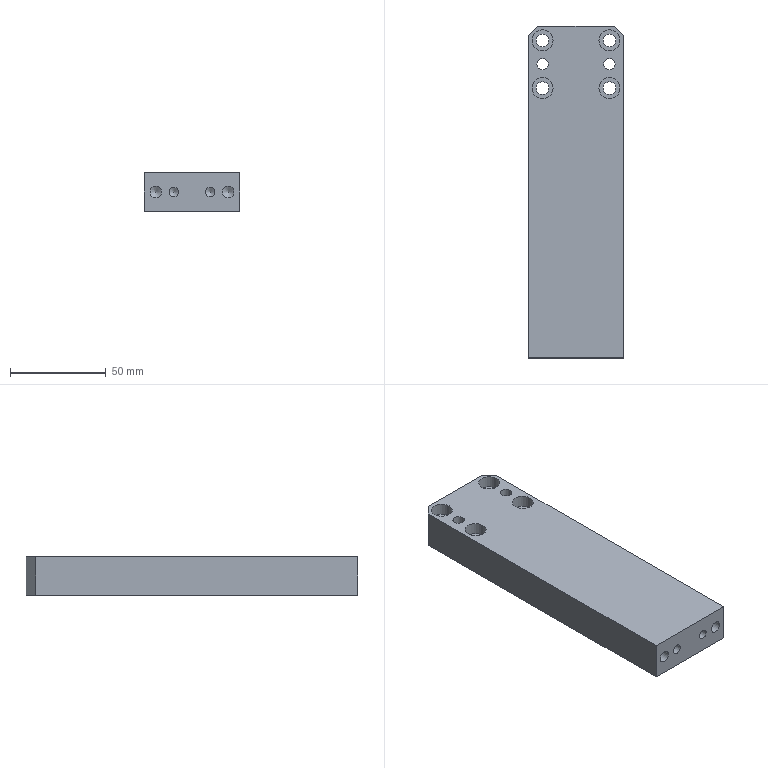Part | NX | features BREP 1 | 1 solid | 30 faces | box 50 x 173.75 x 20 mm | volume 166504 mm3 | cylinder 14 | plane 12 | cone 4 | commonest cylinder face diameters 6 x4 6.6 x4 11 x4 5 x2
STEP:
#1=CARTESIAN_POINT('',(25.,81.875,0.));
#2=VERTEX_POINT('',#1);
#3=CARTESIAN_POINT('',(20.,86.875,0.));
#4=VERTEX_POINT('',#3);
#5=CARTESIAN_POINT('',(25.,81.875,0.));
#6=DIRECTION('',(-0.7071,0.7071,0.));
#7=VECTOR('',#6,1000.);
#8=LINE('',#5,#7);
#9=EDGE_CURVE('',#2,#4,#8,.T.);
#10=ORIENTED_EDGE('',*,*,#9,.F.);
#11=CARTESIAN_POINT('',(25.,-86.875,0.));
#12=VERTEX_POINT('',#11);
#13=CARTESIAN_POINT('',(25.,0.,0.));
#14=DIRECTION('',(0.,1.,0.));
#15=VECTOR('',#14,1000.);
#16=LINE('',#13,#15);
#17=EDGE_CURVE('',#12,#2,#16,.T.);
#18=ORIENTED_EDGE('',*,*,#17,.F.);
#19=CARTESIAN_POINT('',(-25.,-86.875,0.));
#20=VERTEX_POINT('',#19);
#21=CARTESIAN_POINT('',(0.,-86.875,0.));
#22=DIRECTION('',(1.,0.,0.));
#23=VECTOR('',#22,1000.);
#24=LINE('',#21,#23);
#25=EDGE_CURVE('',#20,#12,#24,.T.);
#26=ORIENTED_EDGE('',*,*,#25,.F.);
#27=CARTESIAN_POINT('',(-25.,81.875,0.));
#28=VERTEX_POINT('',#27);
#29=CARTESIAN_POINT('',(-25.,0.,0.));
#30=DIRECTION('',(0.,-1.,0.));
#31=VECTOR('',#30,1000.);
#32=LINE('',#29,#31);
#33=EDGE_CURVE('',#28,#20,#32,.T.);
#34=ORIENTED_EDGE('',*,*,#33,.F.);
#35=CARTESIAN_POINT('',(-20.,86.875,0.));
#36=VERTEX_POINT('',#35);
#37=CARTESIAN_POINT('',(-20.,86.875,0.));
#38=DIRECTION('',(-0.7071,-0.7071,0.));
#39=VECTOR('',#38,1000.);
#40=LINE('',#37,#39);
#41=EDGE_CURVE('',#36,#28,#40,.T.);
#42=ORIENTED_EDGE('',*,*,#41,.F.);
#43=CARTESIAN_POINT('',(0.,86.875,0.));
#44=DIRECTION('',(-1.,0.,0.));
#45=VECTOR('',#44,1000.);
#46=LINE('',#43,#45);
#47=EDGE_CURVE('',#4,#36,#46,.T.);
#48=ORIENTED_EDGE('',*,*,#47,.F.);
#49=EDGE_LOOP('',(#10,#18,#26,#34,#42,#48));
#50=FACE_BOUND('',#49,.T.);
#51=CARTESIAN_POINT('',(14.5,66.875,0.));
#52=VERTEX_POINT('',#51);
#53=CARTESIAN_POINT('',(17.5,66.875,0.));
#54=DIRECTION('',(0.,0.,-1.));
#55=DIRECTION('',(-1.,0.,0.));
#56=AXIS2_PLACEMENT_3D('',#53,#54,#55);
#57=CIRCLE('',#56,3.);
#58=EDGE_CURVE('',#52,#52,#57,.T.);
#59=ORIENTED_EDGE('',*,*,#58,.F.);
#60=EDGE_LOOP('',(#59));
#61=FACE_BOUND('',#60,.T.);
#62=CARTESIAN_POINT('',(-20.5,66.875,0.));
#63=VERTEX_POINT('',#62);
#64=CARTESIAN_POINT('',(-17.5,66.875,0.));
#65=DIRECTION('',(0.,0.,-1.));
#66=DIRECTION('',(-1.,0.,0.));
#67=AXIS2_PLACEMENT_3D('',#64,#65,#66);
#68=CIRCLE('',#67,3.);
#69=EDGE_CURVE('',#63,#63,#68,.T.);
#70=ORIENTED_EDGE('',*,*,#69,.F.);
#71=EDGE_LOOP('',(#70));
#72=FACE_BOUND('',#71,.T.);
#73=CARTESIAN_POINT('',(20.8,54.375,0.));
#74=VERTEX_POINT('',#73);
#75=CARTESIAN_POINT('',(17.5,54.375,0.));
#76=DIRECTION('',(0.,0.,-1.));
#77=DIRECTION('',(1.,0.,0.));
#78=AXIS2_PLACEMENT_3D('',#75,#76,#77);
#79=CIRCLE('',#78,3.3);
#80=EDGE_CURVE('',#74,#74,#79,.T.);
#81=ORIENTED_EDGE('',*,*,#80,.F.);
#82=EDGE_LOOP('',(#81));
#83=FACE_BOUND('',#82,.T.);
#84=CARTESIAN_POINT('',(20.8,79.375,0.));
#85=VERTEX_POINT('',#84);
#86=CARTESIAN_POINT('',(17.5,79.375,0.));
#87=DIRECTION('',(0.,0.,-1.));
#88=DIRECTION('',(1.,0.,0.));
#89=AXIS2_PLACEMENT_3D('',#86,#87,#88);
#90=CIRCLE('',#89,3.3);
#91=EDGE_CURVE('',#85,#85,#90,.T.);
#92=ORIENTED_EDGE('',*,*,#91,.F.);
#93=EDGE_LOOP('',(#92));
#94=FACE_BOUND('',#93,.T.);
#95=CARTESIAN_POINT('',(-14.2,54.375,0.));
#96=VERTEX_POINT('',#95);
#97=CARTESIAN_POINT('',(-17.5,54.375,0.));
#98=DIRECTION('',(0.,0.,-1.));
#99=DIRECTION('',(1.,0.,0.));
#100=AXIS2_PLACEMENT_3D('',#97,#98,#99);
#101=CIRCLE('',#100,3.3);
#102=EDGE_CURVE('',#96,#96,#101,.T.);
#103=ORIENTED_EDGE('',*,*,#102,.F.);
#104=EDGE_LOOP('',(#103));
#105=FACE_BOUND('',#104,.T.);
#106=CARTESIAN_POINT('',(-14.2,79.375,0.));
#107=VERTEX_POINT('',#106);
#108=CARTESIAN_POINT('',(-17.5,79.375,0.));
#109=DIRECTION('',(0.,0.,-1.));
#110=DIRECTION('',(1.,0.,0.));
#111=AXIS2_PLACEMENT_3D('',#108,#109,#110);
#112=CIRCLE('',#111,3.3);
#113=EDGE_CURVE('',#107,#107,#112,.T.);
#114=ORIENTED_EDGE('',*,*,#113,.F.);
#115=EDGE_LOOP('',(#114));
#116=FACE_BOUND('',#115,.T.);
#117=CARTESIAN_POINT('',(0.,0.,0.));
#118=DIRECTION('',(0.,0.,1.));
#119=DIRECTION('',(-1.,0.,0.));
#120=AXIS2_PLACEMENT_3D('',#117,#118,#119);
#121=PLANE('',#120);
#122=ADVANCED_FACE('',(#50,#61,#72,#83,#94,#105,#116),#121,.F.);
#123=CARTESIAN_POINT('',(20.,86.875,20.));
#124=VERTEX_POINT('',#123);
#125=CARTESIAN_POINT('',(20.,86.875,20.));
#126=DIRECTION('',(0.,0.,1.));
#127=VECTOR('',#126,1000.);
#128=LINE('',#125,#127);
#129=EDGE_CURVE('',#4,#124,#128,.T.);
#130=ORIENTED_EDGE('',*,*,#129,.F.);
#131=ORIENTED_EDGE('',*,*,#47,.T.);
#132=CARTESIAN_POINT('',(-20.,86.875,20.));
#133=VERTEX_POINT('',#132);
#134=CARTESIAN_POINT('',(-20.,86.875,20.));
#135=DIRECTION('',(0.,0.,-1.));
#136=VECTOR('',#135,1000.);
#137=LINE('',#134,#136);
#138=EDGE_CURVE('',#133,#36,#137,.T.);
#139=ORIENTED_EDGE('',*,*,#138,.F.);
#140=CARTESIAN_POINT('',(-25.,86.875,20.));
#141=DIRECTION('',(-1.,0.,0.));
#142=VECTOR('',#141,1000.);
#143=LINE('',#140,#142);
#144=EDGE_CURVE('',#124,#133,#143,.T.);
#145=ORIENTED_EDGE('',*,*,#144,.F.);
#146=EDGE_LOOP('',(#130,#131,#139,#145));
#147=FACE_BOUND('',#146,.T.);
#148=CARTESIAN_POINT('',(-25.,86.875,20.));
#149=DIRECTION('',(0.,-1.,0.));
#150=DIRECTION('',(0.,0.,1.));
#151=AXIS2_PLACEMENT_3D('',#148,#149,#150);
#152=PLANE('',#151);
#153=ADVANCED_FACE('',(#147),#152,.F.);
#154=CARTESIAN_POINT('',(25.,81.875,20.));
#155=VERTEX_POINT('',#154);
#156=CARTESIAN_POINT('',(25.,81.875,20.));
#157=DIRECTION('',(0.,0.,1.));
#158=VECTOR('',#157,1000.);
#159=LINE('',#156,#158);
#160=EDGE_CURVE('',#2,#155,#159,.T.);
#161=ORIENTED_EDGE('',*,*,#160,.F.);
#162=ORIENTED_EDGE('',*,*,#9,.T.);
#163=ORIENTED_EDGE('',*,*,#129,.T.);
#164=CARTESIAN_POINT('',(20.,86.875,20.));
#165=DIRECTION('',(-0.7071,0.7071,0.));
#166=VECTOR('',#165,1000.);
#167=LINE('',#164,#166);
#168=EDGE_CURVE('',#155,#124,#167,.T.);
#169=ORIENTED_EDGE('',*,*,#168,.F.);
#170=EDGE_LOOP('',(#161,#162,#163,#169));
#171=FACE_BOUND('',#170,.T.);
#172=CARTESIAN_POINT('',(20.,86.875,20.));
#173=DIRECTION('',(-0.7071,-0.7071,0.));
#174=DIRECTION('',(-0.7071,0.7071,0.));
#175=AXIS2_PLACEMENT_3D('',#172,#173,#174);
#176=PLANE('',#175);
#177=ADVANCED_FACE('',(#171),#176,.F.);
#178=ORIENTED_EDGE('',*,*,#160,.T.);
#179=CARTESIAN_POINT('',(25.,-86.875,20.));
#180=VERTEX_POINT('',#179);
#181=CARTESIAN_POINT('',(25.,86.875,20.));
#182=DIRECTION('',(0.,1.,0.));
#183=VECTOR('',#182,1000.);
#184=LINE('',#181,#183);
#185=EDGE_CURVE('',#180,#155,#184,.T.);
#186=ORIENTED_EDGE('',*,*,#185,.F.);
#187=CARTESIAN_POINT('',(25.,-86.875,20.));
#188=DIRECTION('',(0.,0.,1.));
#189=VECTOR('',#188,1000.);
#190=LINE('',#187,#189);
#191=EDGE_CURVE('',#12,#180,#190,.T.);
#192=ORIENTED_EDGE('',*,*,#191,.F.);
#193=ORIENTED_EDGE('',*,*,#17,.T.);
#194=EDGE_LOOP('',(#178,#186,#192,#193));
#195=FACE_BOUND('',#194,.T.);
#196=CARTESIAN_POINT('',(25.,86.875,20.));
#197=DIRECTION('',(-1.,0.,0.));
#198=DIRECTION('',(0.,1.,0.));
#199=AXIS2_PLACEMENT_3D('',#196,#197,#198);
#200=PLANE('',#199);
#201=ADVANCED_FACE('',(#195),#200,.F.);
#202=ORIENTED_EDGE('',*,*,#191,.T.);
#203=CARTESIAN_POINT('',(-25.,-86.875,20.));
#204=VERTEX_POINT('',#203);
#205=CARTESIAN_POINT('',(-25.,-86.875,20.));
#206=DIRECTION('',(1.,0.,0.));
#207=VECTOR('',#206,1000.);
#208=LINE('',#205,#207);
#209=EDGE_CURVE('',#204,#180,#208,.T.);
#210=ORIENTED_EDGE('',*,*,#209,.F.);
#211=CARTESIAN_POINT('',(-25.,-86.875,20.));
#212=DIRECTION('',(0.,0.,1.));
#213=VECTOR('',#212,1000.);
#214=LINE('',#211,#213);
#215=EDGE_CURVE('',#20,#204,#214,.T.);
#216=ORIENTED_EDGE('',*,*,#215,.F.);
#217=ORIENTED_EDGE('',*,*,#25,.T.);
#218=EDGE_LOOP('',(#202,#210,#216,#217));
#219=FACE_BOUND('',#218,.T.);
#220=CARTESIAN_POINT('',(19.,-86.875,7.));
#221=VERTEX_POINT('',#220);
#222=CARTESIAN_POINT('',(19.,-86.875,10.));
#223=DIRECTION('',(0.,-1.,0.));
#224=DIRECTION('',(0.,0.,-1.));
#225=AXIS2_PLACEMENT_3D('',#222,#223,#224);
#226=CIRCLE('',#225,3.);
#227=EDGE_CURVE('',#221,#221,#226,.T.);
#228=ORIENTED_EDGE('',*,*,#227,.F.);
#229=EDGE_LOOP('',(#228));
#230=FACE_BOUND('',#229,.T.);
#231=CARTESIAN_POINT('',(-19.,-86.875,7.));
#232=VERTEX_POINT('',#231);
#233=CARTESIAN_POINT('',(-19.,-86.875,10.));
#234=DIRECTION('',(0.,-1.,0.));
#235=DIRECTION('',(0.,0.,-1.));
#236=AXIS2_PLACEMENT_3D('',#233,#234,#235);
#237=CIRCLE('',#236,3.);
#238=EDGE_CURVE('',#232,#232,#237,.T.);
#239=ORIENTED_EDGE('',*,*,#238,.F.);
#240=EDGE_LOOP('',(#239));
#241=FACE_BOUND('',#240,.T.);
#242=CARTESIAN_POINT('',(9.5,-86.875,7.5));
#243=VERTEX_POINT('',#242);
#244=CARTESIAN_POINT('',(9.5,-86.875,10.));
#245=DIRECTION('',(0.,-1.,0.));
#246=DIRECTION('',(0.,0.,-1.));
#247=AXIS2_PLACEMENT_3D('',#244,#245,#246);
#248=CIRCLE('',#247,2.5);
#249=EDGE_CURVE('',#243,#243,#248,.T.);
#250=ORIENTED_EDGE('',*,*,#249,.F.);
#251=EDGE_LOOP('',(#250));
#252=FACE_BOUND('',#251,.T.);
#253=CARTESIAN_POINT('',(-9.5,-86.875,7.5));
#254=VERTEX_POINT('',#253);
#255=CARTESIAN_POINT('',(-9.5,-86.875,10.));
#256=DIRECTION('',(0.,-1.,0.));
#257=DIRECTION('',(0.,0.,-1.));
#258=AXIS2_PLACEMENT_3D('',#255,#256,#257);
#259=CIRCLE('',#258,2.5);
#260=EDGE_CURVE('',#254,#254,#259,.T.);
#261=ORIENTED_EDGE('',*,*,#260,.F.);
#262=EDGE_LOOP('',(#261));
#263=FACE_BOUND('',#262,.T.);
#264=CARTESIAN_POINT('',(-25.,-86.875,20.));
#265=DIRECTION('',(0.,1.,0.));
#266=DIRECTION('',(0.,0.,-1.));
#267=AXIS2_PLACEMENT_3D('',#264,#265,#266);
#268=PLANE('',#267);
#269=ADVANCED_FACE('',(#219,#230,#241,#252,#263),#268,.F.);
#270=CARTESIAN_POINT('',(-25.,81.875,20.));
#271=VERTEX_POINT('',#270);
#272=CARTESIAN_POINT('',(-25.,81.875,20.));
#273=DIRECTION('',(0.,0.,1.));
#274=VECTOR('',#273,1000.);
#275=LINE('',#272,#274);
#276=EDGE_CURVE('',#28,#271,#275,.T.);
#277=ORIENTED_EDGE('',*,*,#276,.F.);
#278=ORIENTED_EDGE('',*,*,#33,.T.);
#279=ORIENTED_EDGE('',*,*,#215,.T.);
#280=CARTESIAN_POINT('',(-25.,86.875,20.));
#281=DIRECTION('',(0.,-1.,0.));
#282=VECTOR('',#281,1000.);
#283=LINE('',#280,#282);
#284=EDGE_CURVE('',#271,#204,#283,.T.);
#285=ORIENTED_EDGE('',*,*,#284,.F.);
#286=EDGE_LOOP('',(#277,#278,#279,#285));
#287=FACE_BOUND('',#286,.T.);
#288=CARTESIAN_POINT('',(-25.,86.875,20.));
#289=DIRECTION('',(1.,0.,0.));
#290=DIRECTION('',(0.,-1.,0.));
#291=AXIS2_PLACEMENT_3D('',#288,#289,#290);
#292=PLANE('',#291);
#293=ADVANCED_FACE('',(#287),#292,.F.);
#294=ORIENTED_EDGE('',*,*,#138,.T.);
#295=ORIENTED_EDGE('',*,*,#41,.T.);
#296=ORIENTED_EDGE('',*,*,#276,.T.);
#297=CARTESIAN_POINT('',(-25.,81.875,20.));
#298=DIRECTION('',(-0.7071,-0.7071,0.));
#299=VECTOR('',#298,1000.);
#300=LINE('',#297,#299);
#301=EDGE_CURVE('',#133,#271,#300,.T.);
#302=ORIENTED_EDGE('',*,*,#301,.F.);
#303=EDGE_LOOP('',(#294,#295,#296,#302));
#304=FACE_BOUND('',#303,.T.);
#305=CARTESIAN_POINT('',(-25.,81.875,20.));
#306=DIRECTION('',(0.7071,-0.7071,0.));
#307=DIRECTION('',(-0.7071,-0.7071,0.));
#308=AXIS2_PLACEMENT_3D('',#305,#306,#307);
#309=PLANE('',#308);
#310=ADVANCED_FACE('',(#304),#309,.F.);
#311=CARTESIAN_POINT('',(14.5,66.875,20.));
#312=VERTEX_POINT('',#311);
#313=CARTESIAN_POINT('',(17.5,66.875,20.));
#314=DIRECTION('',(0.,0.,-1.));
#315=DIRECTION('',(-1.,0.,0.));
#316=AXIS2_PLACEMENT_3D('',#313,#314,#315);
#317=CIRCLE('',#316,3.);
#318=EDGE_CURVE('',#312,#312,#317,.T.);
#319=ORIENTED_EDGE('',*,*,#318,.F.);
#320=EDGE_LOOP('',(#319));
#321=FACE_BOUND('',#320,.T.);
#322=ORIENTED_EDGE('',*,*,#58,.T.);
#323=EDGE_LOOP('',(#322));
#324=FACE_BOUND('',#323,.T.);
#325=CARTESIAN_POINT('',(17.5,66.875,0.));
#326=DIRECTION('',(0.,0.,-1.));
#327=DIRECTION('',(1.,0.,0.));
#328=AXIS2_PLACEMENT_3D('',#325,#326,#327);
#329=CYLINDRICAL_SURFACE('',#328,3.);
#330=ADVANCED_FACE('',(#321,#324),#329,.F.);
#331=CARTESIAN_POINT('',(-20.5,66.875,20.));
#332=VERTEX_POINT('',#331);
#333=CARTESIAN_POINT('',(-17.5,66.875,20.));
#334=DIRECTION('',(0.,0.,-1.));
#335=DIRECTION('',(-1.,0.,0.));
#336=AXIS2_PLACEMENT_3D('',#333,#334,#335);
#337=CIRCLE('',#336,3.);
#338=EDGE_CURVE('',#332,#332,#337,.T.);
#339=ORIENTED_EDGE('',*,*,#338,.F.);
#340=EDGE_LOOP('',(#339));
#341=FACE_BOUND('',#340,.T.);
#342=ORIENTED_EDGE('',*,*,#69,.T.);
#343=EDGE_LOOP('',(#342));
#344=FACE_BOUND('',#343,.T.);
#345=CARTESIAN_POINT('',(-17.5,66.875,0.));
#346=DIRECTION('',(0.,0.,-1.));
#347=DIRECTION('',(1.,0.,0.));
#348=AXIS2_PLACEMENT_3D('',#345,#346,#347);
#349=CYLINDRICAL_SURFACE('',#348,3.);
#350=ADVANCED_FACE('',(#341,#344),#349,.F.);
#351=ORIENTED_EDGE('',*,*,#80,.T.);
#352=EDGE_LOOP('',(#351));
#353=FACE_BOUND('',#352,.T.);
#354=CARTESIAN_POINT('',(20.8,54.375,13.6));
#355=VERTEX_POINT('',#354);
#356=CARTESIAN_POINT('',(17.5,54.375,13.6));
#357=DIRECTION('',(0.,0.,-1.));
#358=DIRECTION('',(1.,0.,0.));
#359=AXIS2_PLACEMENT_3D('',#356,#357,#358);
#360=CIRCLE('',#359,3.3);
#361=EDGE_CURVE('',#355,#355,#360,.T.);
#362=ORIENTED_EDGE('',*,*,#361,.F.);
#363=EDGE_LOOP('',(#362));
#364=FACE_BOUND('',#363,.T.);
#365=CARTESIAN_POINT('',(17.5,54.375,20.));
#366=DIRECTION('',(0.,0.,1.));
#367=DIRECTION('',(-1.,0.,0.));
#368=AXIS2_PLACEMENT_3D('',#365,#366,#367);
#369=CYLINDRICAL_SURFACE('',#368,3.3);
#370=ADVANCED_FACE('',(#353,#364),#369,.F.);
#371=ORIENTED_EDGE('',*,*,#91,.T.);
#372=EDGE_LOOP('',(#371));
#373=FACE_BOUND('',#372,.T.);
#374=CARTESIAN_POINT('',(20.8,79.375,13.6));
#375=VERTEX_POINT('',#374);
#376=CARTESIAN_POINT('',(17.5,79.375,13.6));
#377=DIRECTION('',(0.,0.,-1.));
#378=DIRECTION('',(1.,0.,0.));
#379=AXIS2_PLACEMENT_3D('',#376,#377,#378);
#380=CIRCLE('',#379,3.3);
#381=EDGE_CURVE('',#375,#375,#380,.T.);
#382=ORIENTED_EDGE('',*,*,#381,.F.);
#383=EDGE_LOOP('',(#382));
#384=FACE_BOUND('',#383,.T.);
#385=CARTESIAN_POINT('',(17.5,79.375,20.));
#386=DIRECTION('',(0.,0.,1.));
#387=DIRECTION('',(-1.,0.,0.));
#388=AXIS2_PLACEMENT_3D('',#385,#386,#387);
#389=CYLINDRICAL_SURFACE('',#388,3.3);
#390=ADVANCED_FACE('',(#373,#384),#389,.F.);
#391=ORIENTED_EDGE('',*,*,#102,.T.);
#392=EDGE_LOOP('',(#391));
#393=FACE_BOUND('',#392,.T.);
#394=CARTESIAN_POINT('',(-14.2,54.375,13.6));
#395=VERTEX_POINT('',#394);
#396=CARTESIAN_POINT('',(-17.5,54.375,13.6));
#397=DIRECTION('',(0.,0.,-1.));
#398=DIRECTION('',(1.,0.,0.));
#399=AXIS2_PLACEMENT_3D('',#396,#397,#398);
#400=CIRCLE('',#399,3.3);
#401=EDGE_CURVE('',#395,#395,#400,.T.);
#402=ORIENTED_EDGE('',*,*,#401,.F.);
#403=EDGE_LOOP('',(#402));
#404=FACE_BOUND('',#403,.T.);
#405=CARTESIAN_POINT('',(-17.5,54.375,20.));
#406=DIRECTION('',(0.,0.,1.));
#407=DIRECTION('',(-1.,0.,0.));
#408=AXIS2_PLACEMENT_3D('',#405,#406,#407);
#409=CYLINDRICAL_SURFACE('',#408,3.3);
#410=ADVANCED_FACE('',(#393,#404),#409,.F.);
#411=ORIENTED_EDGE('',*,*,#113,.T.);
#412=EDGE_LOOP('',(#411));
#413=FACE_BOUND('',#412,.T.);
#414=CARTESIAN_POINT('',(-14.2,79.375,13.6));
#415=VERTEX_POINT('',#414);
#416=CARTESIAN_POINT('',(-17.5,79.375,13.6));
#417=DIRECTION('',(0.,0.,-1.));
#418=DIRECTION('',(1.,0.,0.));
#419=AXIS2_PLACEMENT_3D('',#416,#417,#418);
#420=CIRCLE('',#419,3.3);
#421=EDGE_CURVE('',#415,#415,#420,.T.);
#422=ORIENTED_EDGE('',*,*,#421,.F.);
#423=EDGE_LOOP('',(#422));
#424=FACE_BOUND('',#423,.T.);
#425=CARTESIAN_POINT('',(-17.5,79.375,20.));
#426=DIRECTION('',(0.,0.,1.));
#427=DIRECTION('',(-1.,0.,0.));
#428=AXIS2_PLACEMENT_3D('',#425,#426,#427);
#429=CYLINDRICAL_SURFACE('',#428,3.3);
#430=ADVANCED_FACE('',(#413,#424),#429,.F.);
#431=ORIENTED_EDGE('',*,*,#284,.T.);
#432=ORIENTED_EDGE('',*,*,#209,.T.);
#433=ORIENTED_EDGE('',*,*,#185,.T.);
#434=ORIENTED_EDGE('',*,*,#168,.T.);
#435=ORIENTED_EDGE('',*,*,#144,.T.);
#436=ORIENTED_EDGE('',*,*,#301,.T.);
#437=EDGE_LOOP('',(#431,#432,#433,#434,#435,#436));
#438=FACE_BOUND('',#437,.T.);
#439=ORIENTED_EDGE('',*,*,#318,.T.);
#440=EDGE_LOOP('',(#439));
#441=FACE_BOUND('',#440,.T.);
#442=ORIENTED_EDGE('',*,*,#338,.T.);
#443=EDGE_LOOP('',(#442));
#444=FACE_BOUND('',#443,.T.);
#445=CARTESIAN_POINT('',(23.,54.375,20.));
#446=VERTEX_POINT('',#445);
#447=CARTESIAN_POINT('',(17.5,54.375,20.));
#448=DIRECTION('',(0.,0.,-1.));
#449=DIRECTION('',(1.,0.,0.));
#450=AXIS2_PLACEMENT_3D('',#447,#448,#449);
#451=CIRCLE('',#450,5.5);
#452=EDGE_CURVE('',#446,#446,#451,.T.);
#453=ORIENTED_EDGE('',*,*,#452,.T.);
#454=EDGE_LOOP('',(#453));
#455=FACE_BOUND('',#454,.T.);
#456=CARTESIAN_POINT('',(23.,79.375,20.));
#457=VERTEX_POINT('',#456);
#458=CARTESIAN_POINT('',(17.5,79.375,20.));
#459=DIRECTION('',(0.,0.,-1.));
#460=DIRECTION('',(1.,0.,0.));
#461=AXIS2_PLACEMENT_3D('',#458,#459,#460);
#462=CIRCLE('',#461,5.5);
#463=EDGE_CURVE('',#457,#457,#462,.T.);
#464=ORIENTED_EDGE('',*,*,#463,.T.);
#465=EDGE_LOOP('',(#464));
#466=FACE_BOUND('',#465,.T.);
#467=CARTESIAN_POINT('',(-12.,54.375,20.));
#468=VERTEX_POINT('',#467);
#469=CARTESIAN_POINT('',(-17.5,54.375,20.));
#470=DIRECTION('',(0.,0.,-1.));
#471=DIRECTION('',(1.,0.,0.));
#472=AXIS2_PLACEMENT_3D('',#469,#470,#471);
#473=CIRCLE('',#472,5.5);
#474=EDGE_CURVE('',#468,#468,#473,.T.);
#475=ORIENTED_EDGE('',*,*,#474,.T.);
#476=EDGE_LOOP('',(#475));
#477=FACE_BOUND('',#476,.T.);
#478=CARTESIAN_POINT('',(-12.,79.375,20.));
#479=VERTEX_POINT('',#478);
#480=CARTESIAN_POINT('',(-17.5,79.375,20.));
#481=DIRECTION('',(0.,0.,-1.));
#482=DIRECTION('',(1.,0.,0.));
#483=AXIS2_PLACEMENT_3D('',#480,#481,#482);
#484=CIRCLE('',#483,5.5);
#485=EDGE_CURVE('',#479,#479,#484,.T.);
#486=ORIENTED_EDGE('',*,*,#485,.T.);
#487=EDGE_LOOP('',(#486));
#488=FACE_BOUND('',#487,.T.);
#489=CARTESIAN_POINT('',(0.,0.,20.));
#490=DIRECTION('',(0.,0.,1.));
#491=DIRECTION('',(-1.,0.,0.));
#492=AXIS2_PLACEMENT_3D('',#489,#490,#491);
#493=PLANE('',#492);
#494=ADVANCED_FACE('',(#438,#441,#444,#455,#466,#477,#488),#493,.T.);
#495=CARTESIAN_POINT('',(19.,-74.875,7.));
#496=VERTEX_POINT('',#495);
#497=CARTESIAN_POINT('',(19.,-74.875,10.));
#498=DIRECTION('',(0.,-1.,0.));
#499=DIRECTION('',(0.,0.,-1.));
#500=AXIS2_PLACEMENT_3D('',#497,#498,#499);
#501=CIRCLE('',#500,3.);
#502=EDGE_CURVE('',#496,#496,#501,.T.);
#503=ORIENTED_EDGE('',*,*,#502,.F.);
#504=EDGE_LOOP('',(#503));
#505=FACE_BOUND('',#504,.T.);
#506=ORIENTED_EDGE('',*,*,#227,.T.);
#507=EDGE_LOOP('',(#506));
#508=FACE_BOUND('',#507,.T.);
#509=CARTESIAN_POINT('',(19.,-86.875,10.));
#510=DIRECTION('',(0.,-1.,0.));
#511=DIRECTION('',(0.,0.,1.));
#512=AXIS2_PLACEMENT_3D('',#509,#510,#511);
#513=CYLINDRICAL_SURFACE('',#512,3.);
#514=ADVANCED_FACE('',(#505,#508),#513,.F.);
#515=CARTESIAN_POINT('',(-19.,-74.875,7.));
#516=VERTEX_POINT('',#515);
#517=CARTESIAN_POINT('',(-19.,-74.875,10.));
#518=DIRECTION('',(0.,-1.,0.));
#519=DIRECTION('',(0.,0.,-1.));
#520=AXIS2_PLACEMENT_3D('',#517,#518,#519);
#521=CIRCLE('',#520,3.);
#522=EDGE_CURVE('',#516,#516,#521,.T.);
#523=ORIENTED_EDGE('',*,*,#522,.F.);
#524=EDGE_LOOP('',(#523));
#525=FACE_BOUND('',#524,.T.);
#526=ORIENTED_EDGE('',*,*,#238,.T.);
#527=EDGE_LOOP('',(#526));
#528=FACE_BOUND('',#527,.T.);
#529=CARTESIAN_POINT('',(-19.,-86.875,10.));
#530=DIRECTION('',(0.,-1.,0.));
#531=DIRECTION('',(0.,0.,1.));
#532=AXIS2_PLACEMENT_3D('',#529,#530,#531);
#533=CYLINDRICAL_SURFACE('',#532,3.);
#534=ADVANCED_FACE('',(#525,#528),#533,.F.);
#535=CARTESIAN_POINT('',(9.5,-71.875,7.5));
#536=VERTEX_POINT('',#535);
#537=CARTESIAN_POINT('',(9.5,-71.875,10.));
#538=DIRECTION('',(0.,-1.,0.));
#539=DIRECTION('',(0.,0.,-1.));
#540=AXIS2_PLACEMENT_3D('',#537,#538,#539);
#541=CIRCLE('',#540,2.5);
#542=EDGE_CURVE('',#536,#536,#541,.T.);
#543=ORIENTED_EDGE('',*,*,#542,.F.);
#544=EDGE_LOOP('',(#543));
#545=FACE_BOUND('',#544,.T.);
#546=ORIENTED_EDGE('',*,*,#249,.T.);
#547=EDGE_LOOP('',(#546));
#548=FACE_BOUND('',#547,.T.);
#549=CARTESIAN_POINT('',(9.5,-86.875,10.));
#550=DIRECTION('',(0.,-1.,0.));
#551=DIRECTION('',(0.,0.,1.));
#552=AXIS2_PLACEMENT_3D('',#549,#550,#551);
#553=CYLINDRICAL_SURFACE('',#552,2.5);
#554=ADVANCED_FACE('',(#545,#548),#553,.F.);
#555=CARTESIAN_POINT('',(-9.5,-71.875,7.5));
#556=VERTEX_POINT('',#555);
#557=CARTESIAN_POINT('',(-9.5,-71.875,10.));
#558=DIRECTION('',(0.,-1.,0.));
#559=DIRECTION('',(0.,0.,-1.));
#560=AXIS2_PLACEMENT_3D('',#557,#558,#559);
#561=CIRCLE('',#560,2.5);
#562=EDGE_CURVE('',#556,#556,#561,.T.);
#563=ORIENTED_EDGE('',*,*,#562,.F.);
#564=EDGE_LOOP('',(#563));
#565=FACE_BOUND('',#564,.T.);
#566=ORIENTED_EDGE('',*,*,#260,.T.);
#567=EDGE_LOOP('',(#566));
#568=FACE_BOUND('',#567,.T.);
#569=CARTESIAN_POINT('',(-9.5,-86.875,10.));
#570=DIRECTION('',(0.,-1.,0.));
#571=DIRECTION('',(0.,0.,1.));
#572=AXIS2_PLACEMENT_3D('',#569,#570,#571);
#573=CYLINDRICAL_SURFACE('',#572,2.5);
#574=ADVANCED_FACE('',(#565,#568),#573,.F.);
#575=CARTESIAN_POINT('',(23.,54.375,13.6));
#576=VERTEX_POINT('',#575);
#577=CARTESIAN_POINT('',(17.5,54.375,13.6));
#578=DIRECTION('',(0.,0.,-1.));
#579=DIRECTION('',(1.,0.,0.));
#580=AXIS2_PLACEMENT_3D('',#577,#578,#579);
#581=CIRCLE('',#580,5.5);
#582=EDGE_CURVE('',#576,#576,#581,.T.);
#583=ORIENTED_EDGE('',*,*,#582,.F.);
#584=EDGE_LOOP('',(#583));
#585=FACE_BOUND('',#584,.T.);
#586=ORIENTED_EDGE('',*,*,#361,.T.);
#587=EDGE_LOOP('',(#586));
#588=FACE_BOUND('',#587,.T.);
#589=CARTESIAN_POINT('',(20.8,54.375,13.6));
#590=DIRECTION('',(0.,0.,-1.));
#591=DIRECTION('',(1.,0.,0.));
#592=AXIS2_PLACEMENT_3D('',#589,#590,#591);
#593=PLANE('',#592);
#594=ADVANCED_FACE('',(#585,#588),#593,.F.);
#595=CARTESIAN_POINT('',(23.,79.375,13.6));
#596=VERTEX_POINT('',#595);
#597=CARTESIAN_POINT('',(17.5,79.375,13.6));
#598=DIRECTION('',(0.,0.,-1.));
#599=DIRECTION('',(1.,0.,0.));
#600=AXIS2_PLACEMENT_3D('',#597,#598,#599);
#601=CIRCLE('',#600,5.5);
#602=EDGE_CURVE('',#596,#596,#601,.T.);
#603=ORIENTED_EDGE('',*,*,#602,.F.);
#604=EDGE_LOOP('',(#603));
#605=FACE_BOUND('',#604,.T.);
#606=ORIENTED_EDGE('',*,*,#381,.T.);
#607=EDGE_LOOP('',(#606));
#608=FACE_BOUND('',#607,.T.);
#609=CARTESIAN_POINT('',(20.8,79.375,13.6));
#610=DIRECTION('',(0.,0.,-1.));
#611=DIRECTION('',(1.,0.,0.));
#612=AXIS2_PLACEMENT_3D('',#609,#610,#611);
#613=PLANE('',#612);
#614=ADVANCED_FACE('',(#605,#608),#613,.F.);
#615=CARTESIAN_POINT('',(-12.,54.375,13.6));
#616=VERTEX_POINT('',#615);
#617=CARTESIAN_POINT('',(-17.5,54.375,13.6));
#618=DIRECTION('',(0.,0.,-1.));
#619=DIRECTION('',(1.,0.,0.));
#620=AXIS2_PLACEMENT_3D('',#617,#618,#619);
#621=CIRCLE('',#620,5.5);
#622=EDGE_CURVE('',#616,#616,#621,.T.);
#623=ORIENTED_EDGE('',*,*,#622,.F.);
#624=EDGE_LOOP('',(#623));
#625=FACE_BOUND('',#624,.T.);
#626=ORIENTED_EDGE('',*,*,#401,.T.);
#627=EDGE_LOOP('',(#626));
#628=FACE_BOUND('',#627,.T.);
#629=CARTESIAN_POINT('',(-14.2,54.375,13.6));
#630=DIRECTION('',(0.,0.,-1.));
#631=DIRECTION('',(1.,0.,0.));
#632=AXIS2_PLACEMENT_3D('',#629,#630,#631);
#633=PLANE('',#632);
#634=ADVANCED_FACE('',(#625,#628),#633,.F.);
#635=CARTESIAN_POINT('',(-12.,79.375,13.6));
#636=VERTEX_POINT('',#635);
#637=CARTESIAN_POINT('',(-17.5,79.375,13.6));
#638=DIRECTION('',(0.,0.,-1.));
#639=DIRECTION('',(1.,0.,0.));
#640=AXIS2_PLACEMENT_3D('',#637,#638,#639);
#641=CIRCLE('',#640,5.5);
#642=EDGE_CURVE('',#636,#636,#641,.T.);
#643=ORIENTED_EDGE('',*,*,#642,.F.);
#644=EDGE_LOOP('',(#643));
#645=FACE_BOUND('',#644,.T.);
#646=ORIENTED_EDGE('',*,*,#421,.T.);
#647=EDGE_LOOP('',(#646));
#648=FACE_BOUND('',#647,.T.);
#649=CARTESIAN_POINT('',(-14.2,79.375,13.6));
#650=DIRECTION('',(0.,0.,-1.));
#651=DIRECTION('',(1.,0.,0.));
#652=AXIS2_PLACEMENT_3D('',#649,#650,#651);
#653=PLANE('',#652);
#654=ADVANCED_FACE('',(#645,#648),#653,.F.);
#655=ORIENTED_EDGE('',*,*,#452,.F.);
#656=EDGE_LOOP('',(#655));
#657=FACE_BOUND('',#656,.T.);
#658=ORIENTED_EDGE('',*,*,#582,.T.);
#659=EDGE_LOOP('',(#658));
#660=FACE_BOUND('',#659,.T.);
#661=CARTESIAN_POINT('',(17.5,54.375,20.));
#662=DIRECTION('',(0.,0.,1.));
#663=DIRECTION('',(-1.,0.,0.));
#664=AXIS2_PLACEMENT_3D('',#661,#662,#663);
#665=CYLINDRICAL_SURFACE('',#664,5.5);
#666=ADVANCED_FACE('',(#657,#660),#665,.F.);
#667=ORIENTED_EDGE('',*,*,#463,.F.);
#668=EDGE_LOOP('',(#667));
#669=FACE_BOUND('',#668,.T.);
#670=ORIENTED_EDGE('',*,*,#602,.T.);
#671=EDGE_LOOP('',(#670));
#672=FACE_BOUND('',#671,.T.);
#673=CARTESIAN_POINT('',(17.5,79.375,20.));
#674=DIRECTION('',(0.,0.,1.));
#675=DIRECTION('',(-1.,0.,0.));
#676=AXIS2_PLACEMENT_3D('',#673,#674,#675);
#677=CYLINDRICAL_SURFACE('',#676,5.5);
#678=ADVANCED_FACE('',(#669,#672),#677,.F.);
#679=ORIENTED_EDGE('',*,*,#474,.F.);
#680=EDGE_LOOP('',(#679));
#681=FACE_BOUND('',#680,.T.);
#682=ORIENTED_EDGE('',*,*,#622,.T.);
#683=EDGE_LOOP('',(#682));
#684=FACE_BOUND('',#683,.T.);
#685=CARTESIAN_POINT('',(-17.5,54.375,20.));
#686=DIRECTION('',(0.,0.,1.));
#687=DIRECTION('',(-1.,0.,0.));
#688=AXIS2_PLACEMENT_3D('',#685,#686,#687);
#689=CYLINDRICAL_SURFACE('',#688,5.5);
#690=ADVANCED_FACE('',(#681,#684),#689,.F.);
#691=ORIENTED_EDGE('',*,*,#485,.F.);
#692=EDGE_LOOP('',(#691));
#693=FACE_BOUND('',#692,.T.);
#694=ORIENTED_EDGE('',*,*,#642,.T.);
#695=EDGE_LOOP('',(#694));
#696=FACE_BOUND('',#695,.T.);
#697=CARTESIAN_POINT('',(-17.5,79.375,20.));
#698=DIRECTION('',(0.,0.,1.));
#699=DIRECTION('',(-1.,0.,0.));
#700=AXIS2_PLACEMENT_3D('',#697,#698,#699);
#701=CYLINDRICAL_SURFACE('',#700,5.5);
#702=ADVANCED_FACE('',(#693,#696),#701,.F.);
#703=CARTESIAN_POINT('',(19.,-73.072,10.));
#704=VERTEX_POINT('',#703);
#705=VERTEX_LOOP('',#704);
#706=FACE_BOUND('',#705,.T.);
#707=ORIENTED_EDGE('',*,*,#502,.T.);
#708=EDGE_LOOP('',(#707));
#709=FACE_BOUND('',#708,.T.);
#710=CARTESIAN_POINT('',(19.,-74.875,10.));
#711=DIRECTION('',(0.,-1.,0.));
#712=DIRECTION('',(0.,0.,1.));
#713=AXIS2_PLACEMENT_3D('',#710,#711,#712);
#714=CONICAL_SURFACE('',#713,3.,1.03);
#715=ADVANCED_FACE('',(#706,#709),#714,.F.);
#716=CARTESIAN_POINT('',(-19.,-73.072,10.));
#717=VERTEX_POINT('',#716);
#718=VERTEX_LOOP('',#717);
#719=FACE_BOUND('',#718,.T.);
#720=ORIENTED_EDGE('',*,*,#522,.T.);
#721=EDGE_LOOP('',(#720));
#722=FACE_BOUND('',#721,.T.);
#723=CARTESIAN_POINT('',(-19.,-74.875,10.));
#724=DIRECTION('',(0.,-1.,0.));
#725=DIRECTION('',(0.,0.,1.));
#726=AXIS2_PLACEMENT_3D('',#723,#724,#725);
#727=CONICAL_SURFACE('',#726,3.,1.03);
#728=ADVANCED_FACE('',(#719,#722),#727,.F.);
#729=CARTESIAN_POINT('',(9.5,-70.373,10.));
#730=VERTEX_POINT('',#729);
#731=VERTEX_LOOP('',#730);
#732=FACE_BOUND('',#731,.T.);
#733=ORIENTED_EDGE('',*,*,#542,.T.);
#734=EDGE_LOOP('',(#733));
#735=FACE_BOUND('',#734,.T.);
#736=CARTESIAN_POINT('',(9.5,-71.875,10.));
#737=DIRECTION('',(0.,-1.,0.));
#738=DIRECTION('',(0.,0.,1.));
#739=AXIS2_PLACEMENT_3D('',#736,#737,#738);
#740=CONICAL_SURFACE('',#739,2.5,1.03);
#741=ADVANCED_FACE('',(#732,#735),#740,.F.);
#742=CARTESIAN_POINT('',(-9.5,-70.373,10.));
#743=VERTEX_POINT('',#742);
#744=VERTEX_LOOP('',#743);
#745=FACE_BOUND('',#744,.T.);
#746=ORIENTED_EDGE('',*,*,#562,.T.);
#747=EDGE_LOOP('',(#746));
#748=FACE_BOUND('',#747,.T.);
#749=CARTESIAN_POINT('',(-9.5,-71.875,10.));
#750=DIRECTION('',(0.,-1.,0.));
#751=DIRECTION('',(0.,0.,1.));
#752=AXIS2_PLACEMENT_3D('',#749,#750,#751);
#753=CONICAL_SURFACE('',#752,2.5,1.03);
#754=ADVANCED_FACE('',(#745,#748),#753,.F.);
#755=CLOSED_SHELL('',(#122,#153,#177,#201,#269,#293,#310,#330,#350,#370,#390,#410,#430,#494,#514,#534,#554,#574,#594,#614,#634,#654,#666,#678,#690,#702,#715,#728,#741,#754));
#756=MANIFOLD_SOLID_BREP('',#755);
#757=(LENGTH_UNIT()NAMED_UNIT(*)SI_UNIT(.MILLI.,.METRE.));
#758=UNCERTAINTY_MEASURE_WITH_UNIT(LENGTH_MEASURE(0.00001),#757,'','');
#759=(NAMED_UNIT(*)PLANE_ANGLE_UNIT()SI_UNIT($,.RADIAN.));
#760=(NAMED_UNIT(*)SI_UNIT($,.STERADIAN.)SOLID_ANGLE_UNIT());
#761=(GEOMETRIC_REPRESENTATION_CONTEXT(3)GLOBAL_UNCERTAINTY_ASSIGNED_CONTEXT((#758))GLOBAL_UNIT_ASSIGNED_CONTEXT((#757,#759,#760))REPRESENTATION_CONTEXT('',''));
#762=ADVANCED_BREP_SHAPE_REPRESENTATION('',(#756),#761);